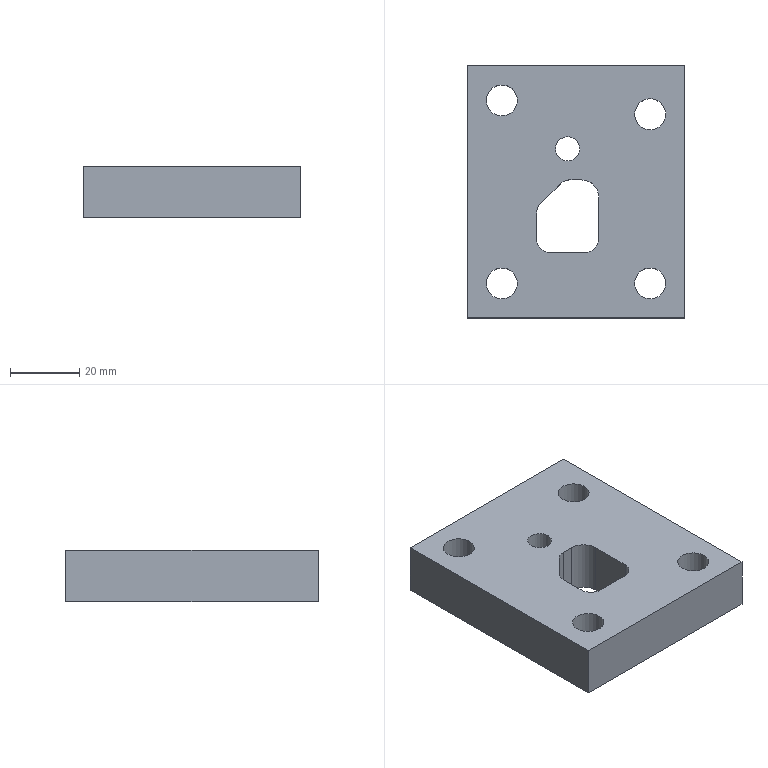Part | STEP file | 1 solid | 21 faces | box 63 x 73 x 15 mm | volume 59595 mm3 | plane 11 | cylinder 9 | spline 1 | commonest cylinder face diameters 9 x4 8 x3 7 x1 10 x1
STEP:
#1=CARTESIAN_POINT('',(-167.586,-61.,-32.));
#2=VERTEX_POINT('',#1);
#3=CARTESIAN_POINT('',(-230.586,-61.,-32.));
#4=VERTEX_POINT('',#3);
#5=CARTESIAN_POINT('',(88.5,-61.,-32.));
#6=DIRECTION('',(-1.,0.,0.));
#7=VECTOR('',#6,1.);
#8=LINE('',#5,#7);
#9=EDGE_CURVE('',#2,#4,#8,.T.);
#10=ORIENTED_EDGE('',*,*,#9,.F.);
#11=CARTESIAN_POINT('',(-167.586,-61.,-47.));
#12=VERTEX_POINT('',#11);
#13=CARTESIAN_POINT('',(-167.586,-61.,-47.));
#14=DIRECTION('',(0.,0.,1.));
#15=VECTOR('',#14,1.);
#16=LINE('',#13,#15);
#17=EDGE_CURVE('',#12,#2,#16,.T.);
#18=ORIENTED_EDGE('',*,*,#17,.F.);
#19=CARTESIAN_POINT('',(-230.586,-61.,-47.));
#20=VERTEX_POINT('',#19);
#21=CARTESIAN_POINT('',(88.5,-61.,-47.));
#22=DIRECTION('',(-1.,0.,0.));
#23=VECTOR('',#22,1.);
#24=LINE('',#21,#23);
#25=EDGE_CURVE('',#12,#20,#24,.T.);
#26=ORIENTED_EDGE('',*,*,#25,.T.);
#27=CARTESIAN_POINT('',(-230.586,-61.,-47.));
#28=DIRECTION('',(0.,0.,1.));
#29=VECTOR('',#28,1.);
#30=LINE('',#27,#29);
#31=EDGE_CURVE('',#20,#4,#30,.T.);
#32=ORIENTED_EDGE('',*,*,#31,.T.);
#33=EDGE_LOOP('',(#10,#18,#26,#32));
#34=FACE_OUTER_BOUND('',#33,.T.);
#35=CARTESIAN_POINT('',(-203.586,-61.,-47.));
#36=DIRECTION('',(0.,1.,0.));
#37=DIRECTION('',(0.,0.,1.));
#38=AXIS2_PLACEMENT_3D('',#35,#36,#37);
#39=PLANE('',#38);
#40=ADVANCED_FACE('',(#34),#39,.T.);
#41=CARTESIAN_POINT('',(-230.586,-134.,-32.));
#42=VERTEX_POINT('',#41);
#43=CARTESIAN_POINT('',(-230.586,-1.,-32.));
#44=DIRECTION('',(0.,-1.,0.));
#45=VECTOR('',#44,1.);
#46=LINE('',#43,#45);
#47=EDGE_CURVE('',#4,#42,#46,.T.);
#48=ORIENTED_EDGE('',*,*,#47,.F.);
#49=ORIENTED_EDGE('',*,*,#31,.F.);
#50=CARTESIAN_POINT('',(-230.586,-134.,-47.));
#51=VERTEX_POINT('',#50);
#52=CARTESIAN_POINT('',(-230.586,-1.,-47.));
#53=DIRECTION('',(0.,-1.,0.));
#54=VECTOR('',#53,1.);
#55=LINE('',#52,#54);
#56=EDGE_CURVE('',#20,#51,#55,.T.);
#57=ORIENTED_EDGE('',*,*,#56,.T.);
#58=CARTESIAN_POINT('',(-230.586,-134.,-47.));
#59=DIRECTION('',(0.,0.,1.));
#60=VECTOR('',#59,1.);
#61=LINE('',#58,#60);
#62=EDGE_CURVE('',#51,#42,#61,.T.);
#63=ORIENTED_EDGE('',*,*,#62,.T.);
#64=EDGE_LOOP('',(#48,#49,#57,#63));
#65=FACE_OUTER_BOUND('',#64,.T.);
#66=CARTESIAN_POINT('',(-230.586,-56.,-47.));
#67=DIRECTION('',(-1.,0.,0.));
#68=DIRECTION('',(0.,0.,1.));
#69=AXIS2_PLACEMENT_3D('',#66,#67,#68);
#70=PLANE('',#69);
#71=ADVANCED_FACE('',(#65),#70,.T.);
#72=CARTESIAN_POINT('',(-167.586,-134.,-32.));
#73=VERTEX_POINT('',#72);
#74=CARTESIAN_POINT('',(-235.586,-134.,-32.));
#75=DIRECTION('',(1.,0.,0.));
#76=VECTOR('',#75,1.);
#77=LINE('',#74,#76);
#78=EDGE_CURVE('',#42,#73,#77,.T.);
#79=ORIENTED_EDGE('',*,*,#78,.F.);
#80=ORIENTED_EDGE('',*,*,#62,.F.);
#81=CARTESIAN_POINT('',(-167.586,-134.,-47.));
#82=VERTEX_POINT('',#81);
#83=CARTESIAN_POINT('',(-235.586,-134.,-47.));
#84=DIRECTION('',(1.,0.,0.));
#85=VECTOR('',#84,1.);
#86=LINE('',#83,#85);
#87=EDGE_CURVE('',#51,#82,#86,.T.);
#88=ORIENTED_EDGE('',*,*,#87,.T.);
#89=CARTESIAN_POINT('',(-167.586,-134.,-47.));
#90=DIRECTION('',(0.,0.,1.));
#91=VECTOR('',#90,1.);
#92=LINE('',#89,#91);
#93=EDGE_CURVE('',#82,#73,#92,.T.);
#94=ORIENTED_EDGE('',*,*,#93,.T.);
#95=EDGE_LOOP('',(#79,#80,#88,#94));
#96=FACE_OUTER_BOUND('',#95,.T.);
#97=CARTESIAN_POINT('',(-235.586,-134.,-47.));
#98=DIRECTION('',(0.,-1.,0.));
#99=DIRECTION('',(0.,0.,-1.));
#100=AXIS2_PLACEMENT_3D('',#97,#98,#99);
#101=PLANE('',#100);
#102=ADVANCED_FACE('',(#96),#101,.T.);
#103=CARTESIAN_POINT('',(-167.586,-139.,-32.));
#104=DIRECTION('',(0.,1.,0.));
#105=VECTOR('',#104,1.);
#106=LINE('',#103,#105);
#107=EDGE_CURVE('',#73,#2,#106,.T.);
#108=ORIENTED_EDGE('',*,*,#107,.F.);
#109=ORIENTED_EDGE('',*,*,#93,.F.);
#110=CARTESIAN_POINT('',(-167.586,-139.,-47.));
#111=DIRECTION('',(0.,1.,0.));
#112=VECTOR('',#111,1.);
#113=LINE('',#110,#112);
#114=EDGE_CURVE('',#82,#12,#113,.T.);
#115=ORIENTED_EDGE('',*,*,#114,.T.);
#116=ORIENTED_EDGE('',*,*,#17,.T.);
#117=EDGE_LOOP('',(#108,#109,#115,#116));
#118=FACE_OUTER_BOUND('',#117,.T.);
#119=CARTESIAN_POINT('',(-167.586,-139.,-47.));
#120=DIRECTION('',(1.,0.,0.));
#121=DIRECTION('',(0.,0.,-1.));
#122=AXIS2_PLACEMENT_3D('',#119,#120,#121);
#123=PLANE('',#122);
#124=ADVANCED_FACE('',(#118),#123,.T.);
#125=CARTESIAN_POINT('',(-173.086,-75.,-47.));
#126=VERTEX_POINT('',#125);
#127=CARTESIAN_POINT('',(-177.586,-75.,-47.));
#128=DIRECTION('',(0.,0.,1.));
#129=DIRECTION('',(1.,0.,0.));
#130=AXIS2_PLACEMENT_3D('',#127,#128,#129);
#131=CIRCLE('',#130,4.5);
#132=EDGE_CURVE('',#126,#126,#131,.T.);
#133=ORIENTED_EDGE('',*,*,#132,.T.);
#134=EDGE_LOOP('',(#133));
#135=FACE_BOUND('',#134,.T.);
#136=CARTESIAN_POINT('',(-216.086,-124.,-47.));
#137=VERTEX_POINT('',#136);
#138=CARTESIAN_POINT('',(-220.586,-124.,-47.));
#139=DIRECTION('',(0.,0.,1.));
#140=DIRECTION('',(1.,0.,0.));
#141=AXIS2_PLACEMENT_3D('',#138,#139,#140);
#142=CIRCLE('',#141,4.5);
#143=EDGE_CURVE('',#137,#137,#142,.T.);
#144=ORIENTED_EDGE('',*,*,#143,.T.);
#145=EDGE_LOOP('',(#144));
#146=FACE_BOUND('',#145,.T.);
#147=CARTESIAN_POINT('',(-225.086,-71.,-47.));
#148=VERTEX_POINT('',#147);
#149=CARTESIAN_POINT('',(-220.586,-71.,-47.));
#150=DIRECTION('',(0.,0.,1.));
#151=DIRECTION('',(-1.,0.,0.));
#152=AXIS2_PLACEMENT_3D('',#149,#150,#151);
#153=CIRCLE('',#152,4.5);
#154=EDGE_CURVE('',#148,#148,#153,.T.);
#155=ORIENTED_EDGE('',*,*,#154,.T.);
#156=EDGE_LOOP('',(#155));
#157=FACE_BOUND('',#156,.T.);
#158=CARTESIAN_POINT('',(-173.086,-124.,-47.));
#159=VERTEX_POINT('',#158);
#160=CARTESIAN_POINT('',(-177.586,-124.,-47.));
#161=DIRECTION('',(0.,0.,1.));
#162=DIRECTION('',(1.,0.,0.));
#163=AXIS2_PLACEMENT_3D('',#160,#161,#162);
#164=CIRCLE('',#163,4.5);
#165=EDGE_CURVE('',#159,#159,#164,.T.);
#166=ORIENTED_EDGE('',*,*,#165,.T.);
#167=EDGE_LOOP('',(#166));
#168=FACE_BOUND('',#167,.T.);
#169=CARTESIAN_POINT('',(-198.,-85.,-47.));
#170=VERTEX_POINT('',#169);
#171=CARTESIAN_POINT('',(-201.5,-85.,-47.));
#172=DIRECTION('',(0.,0.,1.));
#173=DIRECTION('',(1.,0.,0.));
#174=AXIS2_PLACEMENT_3D('',#171,#172,#173);
#175=CIRCLE('',#174,3.5);
#176=EDGE_CURVE('',#170,#170,#175,.T.);
#177=ORIENTED_EDGE('',*,*,#176,.T.);
#178=EDGE_LOOP('',(#177));
#179=FACE_BOUND('',#178,.T.);
#180=ORIENTED_EDGE('',*,*,#25,.F.);
#181=ORIENTED_EDGE('',*,*,#114,.F.);
#182=ORIENTED_EDGE('',*,*,#87,.F.);
#183=ORIENTED_EDGE('',*,*,#56,.F.);
#184=EDGE_LOOP('',(#180,#181,#182,#183));
#185=FACE_BOUND('',#184,.T.);
#186=CARTESIAN_POINT('',(-197.5,-94.,-47.));
#187=VERTEX_POINT('',#186);
#188=CARTESIAN_POINT('',(-200.843,-94.,-47.));
#189=VERTEX_POINT('',#188);
#190=CARTESIAN_POINT('',(88.5,-94.,-47.));
#191=DIRECTION('',(-1.,0.,0.));
#192=VECTOR('',#191,1.);
#193=LINE('',#190,#192);
#194=EDGE_CURVE('',#187,#189,#193,.T.);
#195=ORIENTED_EDGE('',*,*,#194,.T.);
#196=CARTESIAN_POINT('',(-203.672,-95.172,-47.));
#197=VERTEX_POINT('',#196);
#198=CARTESIAN_POINT('',(-200.843,-94.,-47.));
#199=CARTESIAN_POINT('',(-201.108,-94.,-47.));
#200=CARTESIAN_POINT('',(-201.375,-94.026,-47.));
#201=CARTESIAN_POINT('',(-201.635,-94.079,-47.));
#202=CARTESIAN_POINT('',(-202.074,-94.168,-47.));
#203=CARTESIAN_POINT('',(-202.504,-94.334,-47.));
#204=CARTESIAN_POINT('',(-202.889,-94.563,-47.));
#205=CARTESIAN_POINT('',(-203.173,-94.731,-47.));
#206=CARTESIAN_POINT('',(-203.438,-94.938,-47.));
#207=CARTESIAN_POINT('',(-203.672,-95.172,-47.));
#208=B_SPLINE_CURVE_WITH_KNOTS('',3,(#198,#199,#200,#201,#202,#203,#204,#205,#206,#207),.UNSPECIFIED.,.F.,.F.,(4,3,3,4),(0.,0.2529,0.6841,1.),.UNSPECIFIED.);
#209=EDGE_CURVE('',#189,#197,#208,.T.);
#210=ORIENTED_EDGE('',*,*,#209,.T.);
#211=CARTESIAN_POINT('',(-209.328,-100.828,-47.));
#212=VERTEX_POINT('',#211);
#213=CARTESIAN_POINT('',(-10.5,98.,-47.));
#214=DIRECTION('',(-0.7071,-0.7071,0.));
#215=VECTOR('',#214,1.);
#216=LINE('',#213,#215);
#217=EDGE_CURVE('',#197,#212,#216,.T.);
#218=ORIENTED_EDGE('',*,*,#217,.T.);
#219=CARTESIAN_POINT('',(-210.5,-103.657,-47.));
#220=VERTEX_POINT('',#219);
#221=CARTESIAN_POINT('',(-206.5,-103.657,-47.));
#222=DIRECTION('',(0.,0.,1.));
#223=DIRECTION('',(1.,0.,0.));
#224=AXIS2_PLACEMENT_3D('',#221,#222,#223);
#225=CIRCLE('',#224,4.);
#226=EDGE_CURVE('',#212,#220,#225,.T.);
#227=ORIENTED_EDGE('',*,*,#226,.T.);
#228=CARTESIAN_POINT('',(-210.5,-111.,-47.));
#229=VERTEX_POINT('',#228);
#230=CARTESIAN_POINT('',(-210.5,-1.,-47.));
#231=DIRECTION('',(0.,1.,0.));
#232=VECTOR('',#231,1.);
#233=LINE('',#230,#232);
#234=EDGE_CURVE('',#229,#220,#233,.T.);
#235=ORIENTED_EDGE('',*,*,#234,.F.);
#236=CARTESIAN_POINT('',(-206.5,-115.,-47.));
#237=VERTEX_POINT('',#236);
#238=CARTESIAN_POINT('',(-206.5,-111.,-47.));
#239=DIRECTION('',(0.,0.,1.));
#240=DIRECTION('',(1.,0.,0.));
#241=AXIS2_PLACEMENT_3D('',#238,#239,#240);
#242=CIRCLE('',#241,4.);
#243=EDGE_CURVE('',#229,#237,#242,.T.);
#244=ORIENTED_EDGE('',*,*,#243,.T.);
#245=CARTESIAN_POINT('',(-196.5,-115.,-47.));
#246=VERTEX_POINT('',#245);
#247=CARTESIAN_POINT('',(88.5,-115.,-47.));
#248=DIRECTION('',(1.,0.,0.));
#249=VECTOR('',#248,1.);
#250=LINE('',#247,#249);
#251=EDGE_CURVE('',#237,#246,#250,.T.);
#252=ORIENTED_EDGE('',*,*,#251,.T.);
#253=CARTESIAN_POINT('',(-192.5,-111.,-47.));
#254=VERTEX_POINT('',#253);
#255=CARTESIAN_POINT('',(-196.5,-111.,-47.));
#256=DIRECTION('',(0.,0.,1.));
#257=DIRECTION('',(1.,0.,0.));
#258=AXIS2_PLACEMENT_3D('',#255,#256,#257);
#259=CIRCLE('',#258,4.);
#260=EDGE_CURVE('',#246,#254,#259,.T.);
#261=ORIENTED_EDGE('',*,*,#260,.T.);
#262=CARTESIAN_POINT('',(-192.5,-99.,-47.));
#263=VERTEX_POINT('',#262);
#264=CARTESIAN_POINT('',(-192.5,-1.,-47.));
#265=DIRECTION('',(0.,1.,0.));
#266=VECTOR('',#265,1.);
#267=LINE('',#264,#266);
#268=EDGE_CURVE('',#254,#263,#267,.T.);
#269=ORIENTED_EDGE('',*,*,#268,.T.);
#270=CARTESIAN_POINT('',(-197.5,-99.,-47.));
#271=DIRECTION('',(0.,0.,1.));
#272=DIRECTION('',(1.,0.,0.));
#273=AXIS2_PLACEMENT_3D('',#270,#271,#272);
#274=CIRCLE('',#273,5.);
#275=EDGE_CURVE('',#263,#187,#274,.T.);
#276=ORIENTED_EDGE('',*,*,#275,.T.);
#277=EDGE_LOOP('',(#195,#210,#218,#227,#235,#244,#252,#261,#269,#276));
#278=FACE_BOUND('',#277,.T.);
#279=CARTESIAN_POINT('',(88.5,-1.,-47.));
#280=DIRECTION('',(0.,0.,1.));
#281=DIRECTION('',(1.,0.,0.));
#282=AXIS2_PLACEMENT_3D('',#279,#280,#281);
#283=PLANE('',#282);
#284=ADVANCED_FACE('',(#135,#146,#157,#168,#179,#185,#278),#283,.F.);
#285=CARTESIAN_POINT('',(-173.086,-75.,-32.));
#286=VERTEX_POINT('',#285);
#287=CARTESIAN_POINT('',(-177.586,-75.,-32.));
#288=DIRECTION('',(0.,0.,-1.));
#289=DIRECTION('',(1.,0.,0.));
#290=AXIS2_PLACEMENT_3D('',#287,#288,#289);
#291=CIRCLE('',#290,4.5);
#292=EDGE_CURVE('',#286,#286,#291,.T.);
#293=ORIENTED_EDGE('',*,*,#292,.T.);
#294=EDGE_LOOP('',(#293));
#295=FACE_BOUND('',#294,.T.);
#296=CARTESIAN_POINT('',(-216.086,-124.,-32.));
#297=VERTEX_POINT('',#296);
#298=CARTESIAN_POINT('',(-220.586,-124.,-32.));
#299=DIRECTION('',(0.,0.,-1.));
#300=DIRECTION('',(1.,0.,0.));
#301=AXIS2_PLACEMENT_3D('',#298,#299,#300);
#302=CIRCLE('',#301,4.5);
#303=EDGE_CURVE('',#297,#297,#302,.T.);
#304=ORIENTED_EDGE('',*,*,#303,.T.);
#305=EDGE_LOOP('',(#304));
#306=FACE_BOUND('',#305,.T.);
#307=CARTESIAN_POINT('',(-216.086,-71.,-32.));
#308=VERTEX_POINT('',#307);
#309=CARTESIAN_POINT('',(-220.586,-71.,-32.));
#310=DIRECTION('',(0.,0.,1.));
#311=DIRECTION('',(1.,0.,0.));
#312=AXIS2_PLACEMENT_3D('',#309,#310,#311);
#313=CIRCLE('',#312,4.5);
#314=EDGE_CURVE('',#308,#308,#313,.T.);
#315=ORIENTED_EDGE('',*,*,#314,.F.);
#316=EDGE_LOOP('',(#315));
#317=FACE_BOUND('',#316,.T.);
#318=CARTESIAN_POINT('',(-173.086,-124.,-32.));
#319=VERTEX_POINT('',#318);
#320=CARTESIAN_POINT('',(-177.586,-124.,-32.));
#321=DIRECTION('',(0.,0.,1.));
#322=DIRECTION('',(1.,0.,0.));
#323=AXIS2_PLACEMENT_3D('',#320,#321,#322);
#324=CIRCLE('',#323,4.5);
#325=EDGE_CURVE('',#319,#319,#324,.T.);
#326=ORIENTED_EDGE('',*,*,#325,.F.);
#327=EDGE_LOOP('',(#326));
#328=FACE_BOUND('',#327,.T.);
#329=CARTESIAN_POINT('',(-198.,-85.,-32.));
#330=VERTEX_POINT('',#329);
#331=CARTESIAN_POINT('',(-201.5,-85.,-32.));
#332=DIRECTION('',(0.,0.,1.));
#333=DIRECTION('',(1.,0.,0.));
#334=AXIS2_PLACEMENT_3D('',#331,#332,#333);
#335=CIRCLE('',#334,3.5);
#336=EDGE_CURVE('',#330,#330,#335,.T.);
#337=ORIENTED_EDGE('',*,*,#336,.F.);
#338=EDGE_LOOP('',(#337));
#339=FACE_BOUND('',#338,.T.);
#340=ORIENTED_EDGE('',*,*,#9,.T.);
#341=ORIENTED_EDGE('',*,*,#47,.T.);
#342=ORIENTED_EDGE('',*,*,#78,.T.);
#343=ORIENTED_EDGE('',*,*,#107,.T.);
#344=EDGE_LOOP('',(#340,#341,#342,#343));
#345=FACE_BOUND('',#344,.T.);
#346=CARTESIAN_POINT('',(-197.5,-94.,-32.));
#347=VERTEX_POINT('',#346);
#348=CARTESIAN_POINT('',(-200.843,-94.,-32.));
#349=VERTEX_POINT('',#348);
#350=CARTESIAN_POINT('',(88.5,-94.,-32.));
#351=DIRECTION('',(-1.,0.,0.));
#352=VECTOR('',#351,1.);
#353=LINE('',#350,#352);
#354=EDGE_CURVE('',#347,#349,#353,.T.);
#355=ORIENTED_EDGE('',*,*,#354,.F.);
#356=CARTESIAN_POINT('',(-192.5,-99.,-32.));
#357=VERTEX_POINT('',#356);
#358=CARTESIAN_POINT('',(-197.5,-99.,-32.));
#359=DIRECTION('',(0.,0.,1.));
#360=DIRECTION('',(1.,0.,0.));
#361=AXIS2_PLACEMENT_3D('',#358,#359,#360);
#362=CIRCLE('',#361,5.);
#363=EDGE_CURVE('',#357,#347,#362,.T.);
#364=ORIENTED_EDGE('',*,*,#363,.F.);
#365=CARTESIAN_POINT('',(-192.5,-111.,-32.));
#366=VERTEX_POINT('',#365);
#367=CARTESIAN_POINT('',(-192.5,-1.,-32.));
#368=DIRECTION('',(0.,1.,0.));
#369=VECTOR('',#368,1.);
#370=LINE('',#367,#369);
#371=EDGE_CURVE('',#366,#357,#370,.T.);
#372=ORIENTED_EDGE('',*,*,#371,.F.);
#373=CARTESIAN_POINT('',(-196.5,-115.,-32.));
#374=VERTEX_POINT('',#373);
#375=CARTESIAN_POINT('',(-196.5,-111.,-32.));
#376=DIRECTION('',(0.,0.,1.));
#377=DIRECTION('',(1.,0.,0.));
#378=AXIS2_PLACEMENT_3D('',#375,#376,#377);
#379=CIRCLE('',#378,4.);
#380=EDGE_CURVE('',#374,#366,#379,.T.);
#381=ORIENTED_EDGE('',*,*,#380,.F.);
#382=CARTESIAN_POINT('',(-206.5,-115.,-32.));
#383=VERTEX_POINT('',#382);
#384=CARTESIAN_POINT('',(88.5,-115.,-32.));
#385=DIRECTION('',(1.,0.,0.));
#386=VECTOR('',#385,1.);
#387=LINE('',#384,#386);
#388=EDGE_CURVE('',#383,#374,#387,.T.);
#389=ORIENTED_EDGE('',*,*,#388,.F.);
#390=CARTESIAN_POINT('',(-210.5,-111.,-32.));
#391=VERTEX_POINT('',#390);
#392=CARTESIAN_POINT('',(-206.5,-111.,-32.));
#393=DIRECTION('',(0.,0.,1.));
#394=DIRECTION('',(1.,0.,0.));
#395=AXIS2_PLACEMENT_3D('',#392,#393,#394);
#396=CIRCLE('',#395,4.);
#397=EDGE_CURVE('',#391,#383,#396,.T.);
#398=ORIENTED_EDGE('',*,*,#397,.F.);
#399=CARTESIAN_POINT('',(-210.5,-103.657,-32.));
#400=VERTEX_POINT('',#399);
#401=CARTESIAN_POINT('',(-210.5,-1.,-32.));
#402=DIRECTION('',(0.,1.,0.));
#403=VECTOR('',#402,1.);
#404=LINE('',#401,#403);
#405=EDGE_CURVE('',#391,#400,#404,.T.);
#406=ORIENTED_EDGE('',*,*,#405,.T.);
#407=CARTESIAN_POINT('',(-209.328,-100.828,-32.));
#408=VERTEX_POINT('',#407);
#409=CARTESIAN_POINT('',(-206.5,-103.657,-32.));
#410=DIRECTION('',(0.,0.,1.));
#411=DIRECTION('',(1.,0.,0.));
#412=AXIS2_PLACEMENT_3D('',#409,#410,#411);
#413=CIRCLE('',#412,4.);
#414=EDGE_CURVE('',#408,#400,#413,.T.);
#415=ORIENTED_EDGE('',*,*,#414,.F.);
#416=CARTESIAN_POINT('',(-203.672,-95.172,-32.));
#417=VERTEX_POINT('',#416);
#418=CARTESIAN_POINT('',(-10.5,98.,-32.));
#419=DIRECTION('',(-0.7071,-0.7071,0.));
#420=VECTOR('',#419,1.);
#421=LINE('',#418,#420);
#422=EDGE_CURVE('',#417,#408,#421,.T.);
#423=ORIENTED_EDGE('',*,*,#422,.F.);
#424=CARTESIAN_POINT('',(-200.843,-94.,-32.));
#425=CARTESIAN_POINT('',(-201.108,-94.,-32.));
#426=CARTESIAN_POINT('',(-201.375,-94.026,-32.));
#427=CARTESIAN_POINT('',(-201.635,-94.079,-32.));
#428=CARTESIAN_POINT('',(-202.074,-94.168,-32.));
#429=CARTESIAN_POINT('',(-202.504,-94.334,-32.));
#430=CARTESIAN_POINT('',(-202.889,-94.563,-32.));
#431=CARTESIAN_POINT('',(-203.173,-94.731,-32.));
#432=CARTESIAN_POINT('',(-203.438,-94.938,-32.));
#433=CARTESIAN_POINT('',(-203.672,-95.172,-32.));
#434=B_SPLINE_CURVE_WITH_KNOTS('',3,(#424,#425,#426,#427,#428,#429,#430,#431,#432,#433),.UNSPECIFIED.,.F.,.F.,(4,3,3,4),(0.,0.2529,0.6841,1.),.UNSPECIFIED.);
#435=EDGE_CURVE('',#349,#417,#434,.T.);
#436=ORIENTED_EDGE('',*,*,#435,.F.);
#437=EDGE_LOOP('',(#355,#364,#372,#381,#389,#398,#406,#415,#423,#436));
#438=FACE_BOUND('',#437,.T.);
#439=CARTESIAN_POINT('',(88.5,-1.,-32.));
#440=DIRECTION('',(0.,0.,1.));
#441=DIRECTION('',(1.,0.,0.));
#442=AXIS2_PLACEMENT_3D('',#439,#440,#441);
#443=PLANE('',#442);
#444=ADVANCED_FACE('',(#295,#306,#317,#328,#339,#345,#438),#443,.T.);
#445=ORIENTED_EDGE('',*,*,#354,.T.);
#446=CARTESIAN_POINT('',(-200.843,-94.,-47.));
#447=DIRECTION('',(0.,0.,1.));
#448=VECTOR('',#447,1.);
#449=LINE('',#446,#448);
#450=EDGE_CURVE('',#189,#349,#449,.T.);
#451=ORIENTED_EDGE('',*,*,#450,.F.);
#452=ORIENTED_EDGE('',*,*,#194,.F.);
#453=CARTESIAN_POINT('',(-197.5,-94.,-47.));
#454=DIRECTION('',(0.,0.,1.));
#455=VECTOR('',#454,1.);
#456=LINE('',#453,#455);
#457=EDGE_CURVE('',#187,#347,#456,.T.);
#458=ORIENTED_EDGE('',*,*,#457,.T.);
#459=EDGE_LOOP('',(#445,#451,#452,#458));
#460=FACE_OUTER_BOUND('',#459,.T.);
#461=CARTESIAN_POINT('',(-197.5,-94.,-47.));
#462=DIRECTION('',(0.,1.,0.));
#463=DIRECTION('',(0.,0.,1.));
#464=AXIS2_PLACEMENT_3D('',#461,#462,#463);
#465=PLANE('',#464);
#466=ADVANCED_FACE('',(#460),#465,.F.);
#467=ORIENTED_EDGE('',*,*,#363,.T.);
#468=ORIENTED_EDGE('',*,*,#457,.F.);
#469=ORIENTED_EDGE('',*,*,#275,.F.);
#470=CARTESIAN_POINT('',(-192.5,-99.,-47.));
#471=DIRECTION('',(0.,0.,1.));
#472=VECTOR('',#471,1.);
#473=LINE('',#470,#472);
#474=EDGE_CURVE('',#263,#357,#473,.T.);
#475=ORIENTED_EDGE('',*,*,#474,.T.);
#476=EDGE_LOOP('',(#467,#468,#469,#475));
#477=FACE_OUTER_BOUND('',#476,.T.);
#478=CARTESIAN_POINT('',(-197.5,-99.,-47.));
#479=DIRECTION('',(0.,0.,1.));
#480=DIRECTION('',(1.,0.,0.));
#481=AXIS2_PLACEMENT_3D('',#478,#479,#480);
#482=CYLINDRICAL_SURFACE('',#481,5.);
#483=ADVANCED_FACE('',(#477),#482,.F.);
#484=ORIENTED_EDGE('',*,*,#371,.T.);
#485=ORIENTED_EDGE('',*,*,#474,.F.);
#486=ORIENTED_EDGE('',*,*,#268,.F.);
#487=CARTESIAN_POINT('',(-192.5,-111.,-47.));
#488=DIRECTION('',(0.,0.,1.));
#489=VECTOR('',#488,1.);
#490=LINE('',#487,#489);
#491=EDGE_CURVE('',#254,#366,#490,.T.);
#492=ORIENTED_EDGE('',*,*,#491,.T.);
#493=EDGE_LOOP('',(#484,#485,#486,#492));
#494=FACE_OUTER_BOUND('',#493,.T.);
#495=CARTESIAN_POINT('',(-192.5,-111.,-47.));
#496=DIRECTION('',(1.,0.,0.));
#497=DIRECTION('',(0.,0.,-1.));
#498=AXIS2_PLACEMENT_3D('',#495,#496,#497);
#499=PLANE('',#498);
#500=ADVANCED_FACE('',(#494),#499,.F.);
#501=ORIENTED_EDGE('',*,*,#380,.T.);
#502=ORIENTED_EDGE('',*,*,#491,.F.);
#503=ORIENTED_EDGE('',*,*,#260,.F.);
#504=CARTESIAN_POINT('',(-196.5,-115.,-47.));
#505=DIRECTION('',(0.,0.,1.));
#506=VECTOR('',#505,1.);
#507=LINE('',#504,#506);
#508=EDGE_CURVE('',#246,#374,#507,.T.);
#509=ORIENTED_EDGE('',*,*,#508,.T.);
#510=EDGE_LOOP('',(#501,#502,#503,#509));
#511=FACE_OUTER_BOUND('',#510,.T.);
#512=CARTESIAN_POINT('',(-196.5,-111.,-47.));
#513=DIRECTION('',(0.,0.,1.));
#514=DIRECTION('',(1.,0.,0.));
#515=AXIS2_PLACEMENT_3D('',#512,#513,#514);
#516=CYLINDRICAL_SURFACE('',#515,4.);
#517=ADVANCED_FACE('',(#511),#516,.F.);
#518=ORIENTED_EDGE('',*,*,#388,.T.);
#519=ORIENTED_EDGE('',*,*,#508,.F.);
#520=ORIENTED_EDGE('',*,*,#251,.F.);
#521=CARTESIAN_POINT('',(-206.5,-115.,-47.));
#522=DIRECTION('',(0.,0.,1.));
#523=VECTOR('',#522,1.);
#524=LINE('',#521,#523);
#525=EDGE_CURVE('',#237,#383,#524,.T.);
#526=ORIENTED_EDGE('',*,*,#525,.T.);
#527=EDGE_LOOP('',(#518,#519,#520,#526));
#528=FACE_OUTER_BOUND('',#527,.T.);
#529=CARTESIAN_POINT('',(-206.5,-115.,-47.));
#530=DIRECTION('',(0.,-1.,0.));
#531=DIRECTION('',(0.,0.,-1.));
#532=AXIS2_PLACEMENT_3D('',#529,#530,#531);
#533=PLANE('',#532);
#534=ADVANCED_FACE('',(#528),#533,.F.);
#535=ORIENTED_EDGE('',*,*,#397,.T.);
#536=ORIENTED_EDGE('',*,*,#525,.F.);
#537=ORIENTED_EDGE('',*,*,#243,.F.);
#538=CARTESIAN_POINT('',(-210.5,-111.,-47.));
#539=DIRECTION('',(0.,0.,1.));
#540=VECTOR('',#539,1.);
#541=LINE('',#538,#540);
#542=EDGE_CURVE('',#229,#391,#541,.T.);
#543=ORIENTED_EDGE('',*,*,#542,.T.);
#544=EDGE_LOOP('',(#535,#536,#537,#543));
#545=FACE_OUTER_BOUND('',#544,.T.);
#546=CARTESIAN_POINT('',(-206.5,-111.,-47.));
#547=DIRECTION('',(0.,0.,1.));
#548=DIRECTION('',(1.,0.,0.));
#549=AXIS2_PLACEMENT_3D('',#546,#547,#548);
#550=CYLINDRICAL_SURFACE('',#549,4.);
#551=ADVANCED_FACE('',(#545),#550,.F.);
#552=ORIENTED_EDGE('',*,*,#405,.F.);
#553=ORIENTED_EDGE('',*,*,#542,.F.);
#554=ORIENTED_EDGE('',*,*,#234,.T.);
#555=CARTESIAN_POINT('',(-210.5,-103.657,-47.));
#556=DIRECTION('',(0.,0.,1.));
#557=VECTOR('',#556,1.);
#558=LINE('',#555,#557);
#559=EDGE_CURVE('',#220,#400,#558,.T.);
#560=ORIENTED_EDGE('',*,*,#559,.T.);
#561=EDGE_LOOP('',(#552,#553,#554,#560));
#562=FACE_OUTER_BOUND('',#561,.T.);
#563=CARTESIAN_POINT('',(-210.5,-111.,-47.));
#564=DIRECTION('',(1.,0.,0.));
#565=DIRECTION('',(0.,0.,-1.));
#566=AXIS2_PLACEMENT_3D('',#563,#564,#565);
#567=PLANE('',#566);
#568=ADVANCED_FACE('',(#562),#567,.T.);
#569=ORIENTED_EDGE('',*,*,#414,.T.);
#570=ORIENTED_EDGE('',*,*,#559,.F.);
#571=ORIENTED_EDGE('',*,*,#226,.F.);
#572=CARTESIAN_POINT('',(-209.328,-100.828,-47.));
#573=DIRECTION('',(0.,0.,1.));
#574=VECTOR('',#573,1.);
#575=LINE('',#572,#574);
#576=EDGE_CURVE('',#212,#408,#575,.T.);
#577=ORIENTED_EDGE('',*,*,#576,.T.);
#578=EDGE_LOOP('',(#569,#570,#571,#577));
#579=FACE_OUTER_BOUND('',#578,.T.);
#580=CARTESIAN_POINT('',(-206.5,-103.657,-47.));
#581=DIRECTION('',(0.,0.,1.));
#582=DIRECTION('',(1.,0.,0.));
#583=AXIS2_PLACEMENT_3D('',#580,#581,#582);
#584=CYLINDRICAL_SURFACE('',#583,4.);
#585=ADVANCED_FACE('',(#579),#584,.F.);
#586=ORIENTED_EDGE('',*,*,#422,.T.);
#587=ORIENTED_EDGE('',*,*,#576,.F.);
#588=ORIENTED_EDGE('',*,*,#217,.F.);
#589=CARTESIAN_POINT('',(-203.672,-95.172,-47.));
#590=DIRECTION('',(0.,0.,1.));
#591=VECTOR('',#590,1.);
#592=LINE('',#589,#591);
#593=EDGE_CURVE('',#197,#417,#592,.T.);
#594=ORIENTED_EDGE('',*,*,#593,.T.);
#595=EDGE_LOOP('',(#586,#587,#588,#594));
#596=FACE_OUTER_BOUND('',#595,.T.);
#597=CARTESIAN_POINT('',(-203.672,-95.172,-47.));
#598=DIRECTION('',(-0.7071,0.7071,0.));
#599=DIRECTION('',(-0.7071,-0.7071,0.));
#600=AXIS2_PLACEMENT_3D('',#597,#598,#599);
#601=PLANE('',#600);
#602=ADVANCED_FACE('',(#596),#601,.F.);
#603=ORIENTED_EDGE('',*,*,#435,.T.);
#604=ORIENTED_EDGE('',*,*,#593,.F.);
#605=ORIENTED_EDGE('',*,*,#209,.F.);
#606=ORIENTED_EDGE('',*,*,#450,.T.);
#607=EDGE_LOOP('',(#603,#604,#605,#606));
#608=FACE_OUTER_BOUND('',#607,.T.);
#609=CARTESIAN_POINT('',(-203.672,-95.172,-47.));
#610=CARTESIAN_POINT('',(-203.672,-95.172,-32.));
#611=CARTESIAN_POINT('',(-202.941,-94.441,-47.));
#612=CARTESIAN_POINT('',(-202.941,-94.441,-32.));
#613=CARTESIAN_POINT('',(-201.878,-94.,-47.));
#614=CARTESIAN_POINT('',(-201.878,-94.,-32.));
#615=CARTESIAN_POINT('',(-200.843,-94.,-47.));
#616=CARTESIAN_POINT('',(-200.843,-94.,-32.));
#617=B_SPLINE_SURFACE_WITH_KNOTS('',3,1,((#609,#610),(#611,#612),(#613,#614),(#615,#616)),.UNSPECIFIED.,.F.,.F.,.F.,(4,4),(2,2),(0.,1.),(0.,1.),.UNSPECIFIED.);
#618=ADVANCED_FACE('',(#608),#617,.T.);
#619=ORIENTED_EDGE('',*,*,#336,.T.);
#620=EDGE_LOOP('',(#619));
#621=FACE_BOUND('',#620,.T.);
#622=ORIENTED_EDGE('',*,*,#176,.F.);
#623=EDGE_LOOP('',(#622));
#624=FACE_BOUND('',#623,.T.);
#625=CARTESIAN_POINT('',(-201.5,-85.,-31.9));
#626=DIRECTION('',(0.,0.,-1.));
#627=DIRECTION('',(1.,0.,0.));
#628=AXIS2_PLACEMENT_3D('',#625,#626,#627);
#629=CYLINDRICAL_SURFACE('',#628,3.5);
#630=ADVANCED_FACE('',(#621,#624),#629,.F.);
#631=ORIENTED_EDGE('',*,*,#325,.T.);
#632=EDGE_LOOP('',(#631));
#633=FACE_BOUND('',#632,.T.);
#634=ORIENTED_EDGE('',*,*,#165,.F.);
#635=EDGE_LOOP('',(#634));
#636=FACE_BOUND('',#635,.T.);
#637=CARTESIAN_POINT('',(-177.586,-124.,-47.));
#638=DIRECTION('',(0.,0.,1.));
#639=DIRECTION('',(1.,0.,0.));
#640=AXIS2_PLACEMENT_3D('',#637,#638,#639);
#641=CYLINDRICAL_SURFACE('',#640,4.5);
#642=ADVANCED_FACE('',(#633,#636),#641,.F.);
#643=ORIENTED_EDGE('',*,*,#314,.T.);
#644=EDGE_LOOP('',(#643));
#645=FACE_BOUND('',#644,.T.);
#646=ORIENTED_EDGE('',*,*,#154,.F.);
#647=EDGE_LOOP('',(#646));
#648=FACE_BOUND('',#647,.T.);
#649=CARTESIAN_POINT('',(-220.586,-71.,-47.));
#650=DIRECTION('',(0.,0.,1.));
#651=DIRECTION('',(-1.,0.,0.));
#652=AXIS2_PLACEMENT_3D('',#649,#650,#651);
#653=CYLINDRICAL_SURFACE('',#652,4.5);
#654=ADVANCED_FACE('',(#645,#648),#653,.F.);
#655=ORIENTED_EDGE('',*,*,#303,.F.);
#656=EDGE_LOOP('',(#655));
#657=FACE_BOUND('',#656,.T.);
#658=ORIENTED_EDGE('',*,*,#143,.F.);
#659=EDGE_LOOP('',(#658));
#660=FACE_BOUND('',#659,.T.);
#661=CARTESIAN_POINT('',(-220.586,-124.,-47.));
#662=DIRECTION('',(0.,0.,1.));
#663=DIRECTION('',(1.,0.,0.));
#664=AXIS2_PLACEMENT_3D('',#661,#662,#663);
#665=CYLINDRICAL_SURFACE('',#664,4.5);
#666=ADVANCED_FACE('',(#657,#660),#665,.F.);
#667=ORIENTED_EDGE('',*,*,#292,.F.);
#668=EDGE_LOOP('',(#667));
#669=FACE_BOUND('',#668,.T.);
#670=ORIENTED_EDGE('',*,*,#132,.F.);
#671=EDGE_LOOP('',(#670));
#672=FACE_BOUND('',#671,.T.);
#673=CARTESIAN_POINT('',(-177.586,-75.,-47.));
#674=DIRECTION('',(0.,0.,1.));
#675=DIRECTION('',(1.,0.,0.));
#676=AXIS2_PLACEMENT_3D('',#673,#674,#675);
#677=CYLINDRICAL_SURFACE('',#676,4.5);
#678=ADVANCED_FACE('',(#669,#672),#677,.F.);
#679=CLOSED_SHELL('',(#40,#71,#102,#124,#284,#444,#466,#483,#500,#517,#534,#551,#568,#585,#602,#618,#630,#642,#654,#666,#678));
#680=MANIFOLD_SOLID_BREP('',#679);
#681=(LENGTH_UNIT()NAMED_UNIT(*)SI_UNIT(.MILLI.,.METRE.));
#682=UNCERTAINTY_MEASURE_WITH_UNIT(LENGTH_MEASURE(0.0508),#681,'','');
#683=(NAMED_UNIT(*)PLANE_ANGLE_UNIT()SI_UNIT($,.RADIAN.));
#684=PLANE_ANGLE_MEASURE_WITH_UNIT(PLANE_ANGLE_MEASURE(0.01745),#683);
#685=DIMENSIONAL_EXPONENTS(0.,0.,0.,0.,0.,0.,0.);
#686=(CONVERSION_BASED_UNIT('DEGREE',#684)NAMED_UNIT(#685)PLANE_ANGLE_UNIT());
#687=(NAMED_UNIT(*)SI_UNIT($,.STERADIAN.)SOLID_ANGLE_UNIT());
#688=(GEOMETRIC_REPRESENTATION_CONTEXT(3)GLOBAL_UNCERTAINTY_ASSIGNED_CONTEXT((#682))GLOBAL_UNIT_ASSIGNED_CONTEXT((#681,#686,#687))REPRESENTATION_CONTEXT('',''));
#689=ADVANCED_BREP_SHAPE_REPRESENTATION('',(#680),#688);